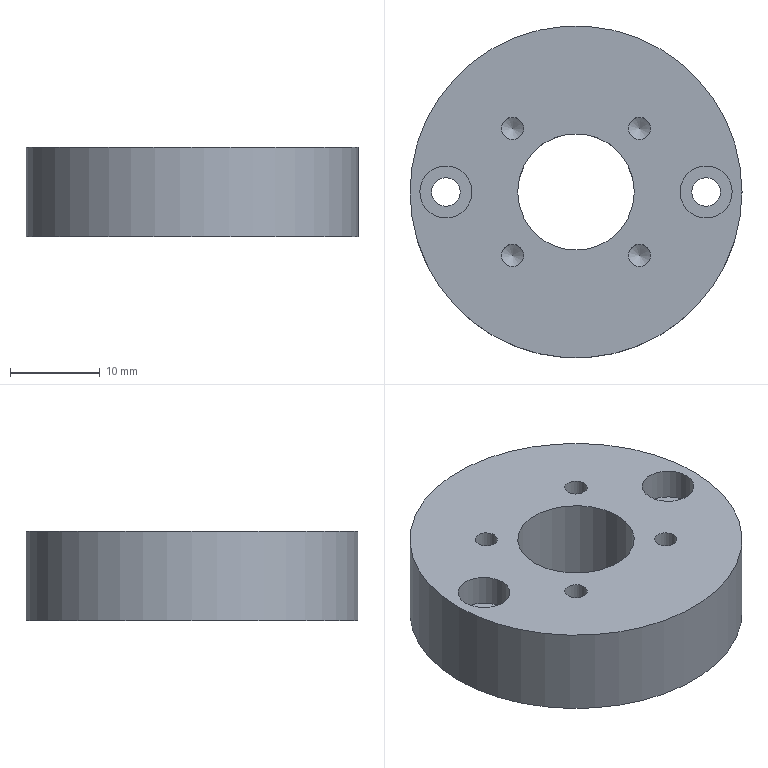Part | NX | 1 solid | 18 faces | box 37 x 37 x 10 mm | volume 8963 mm3 | cylinder 10 | plane 4 | cone 4 | commonest cylinder face diameters 2.5 x4 3.2 x2 5.8 x2 13 x1 37 x1
STEP:
#1=CARTESIAN_POINT('',(18.5,0.,5.));
#2=VERTEX_POINT('',#1);
#3=CARTESIAN_POINT('',(0.,0.,5.));
#4=DIRECTION('',(0.,0.,1.));
#5=DIRECTION('',(1.,0.,0.));
#6=AXIS2_PLACEMENT_3D('',#3,#4,#5);
#7=CIRCLE('',#6,18.5);
#8=EDGE_CURVE('',#2,#2,#7,.T.);
#9=ORIENTED_EDGE('',*,*,#8,.F.);
#10=EDGE_LOOP('',(#9));
#11=FACE_BOUND('',#10,.T.);
#12=CARTESIAN_POINT('',(18.5,0.,-5.));
#13=VERTEX_POINT('',#12);
#14=CARTESIAN_POINT('',(0.,0.,-5.));
#15=DIRECTION('',(0.,0.,1.));
#16=DIRECTION('',(1.,0.,0.));
#17=AXIS2_PLACEMENT_3D('',#14,#15,#16);
#18=CIRCLE('',#17,18.5);
#19=EDGE_CURVE('',#13,#13,#18,.T.);
#20=ORIENTED_EDGE('',*,*,#19,.T.);
#21=EDGE_LOOP('',(#20));
#22=FACE_BOUND('',#21,.T.);
#23=CARTESIAN_POINT('',(0.,0.,5.));
#24=DIRECTION('',(0.,0.,-1.));
#25=DIRECTION('',(-1.,0.,0.));
#26=AXIS2_PLACEMENT_3D('',#23,#24,#25);
#27=CYLINDRICAL_SURFACE('',#26,18.5);
#28=ADVANCED_FACE('',(#11,#22),#27,.T.);
#29=CARTESIAN_POINT('',(6.5,0.,5.));
#30=VERTEX_POINT('',#29);
#31=CARTESIAN_POINT('',(0.,0.,5.));
#32=DIRECTION('',(0.,0.,1.));
#33=DIRECTION('',(1.,0.,0.));
#34=AXIS2_PLACEMENT_3D('',#31,#32,#33);
#35=CIRCLE('',#34,6.5);
#36=EDGE_CURVE('',#30,#30,#35,.T.);
#37=ORIENTED_EDGE('',*,*,#36,.F.);
#38=EDGE_LOOP('',(#37));
#39=FACE_BOUND('',#38,.T.);
#40=CARTESIAN_POINT('',(-5.821,-7.071,5.));
#41=VERTEX_POINT('',#40);
#42=CARTESIAN_POINT('',(-7.071,-7.071,5.));
#43=DIRECTION('',(0.,0.,1.));
#44=DIRECTION('',(1.,0.,0.));
#45=AXIS2_PLACEMENT_3D('',#42,#43,#44);
#46=CIRCLE('',#45,1.25);
#47=EDGE_CURVE('',#41,#41,#46,.T.);
#48=ORIENTED_EDGE('',*,*,#47,.F.);
#49=EDGE_LOOP('',(#48));
#50=FACE_BOUND('',#49,.T.);
#51=CARTESIAN_POINT('',(-5.821,7.071,5.));
#52=VERTEX_POINT('',#51);
#53=CARTESIAN_POINT('',(-7.071,7.071,5.));
#54=DIRECTION('',(0.,0.,1.));
#55=DIRECTION('',(1.,0.,0.));
#56=AXIS2_PLACEMENT_3D('',#53,#54,#55);
#57=CIRCLE('',#56,1.25);
#58=EDGE_CURVE('',#52,#52,#57,.T.);
#59=ORIENTED_EDGE('',*,*,#58,.F.);
#60=EDGE_LOOP('',(#59));
#61=FACE_BOUND('',#60,.T.);
#62=CARTESIAN_POINT('',(8.321,-7.071,5.));
#63=VERTEX_POINT('',#62);
#64=CARTESIAN_POINT('',(7.071,-7.071,5.));
#65=DIRECTION('',(0.,0.,1.));
#66=DIRECTION('',(1.,0.,0.));
#67=AXIS2_PLACEMENT_3D('',#64,#65,#66);
#68=CIRCLE('',#67,1.25);
#69=EDGE_CURVE('',#63,#63,#68,.T.);
#70=ORIENTED_EDGE('',*,*,#69,.F.);
#71=EDGE_LOOP('',(#70));
#72=FACE_BOUND('',#71,.T.);
#73=CARTESIAN_POINT('',(8.321,7.071,5.));
#74=VERTEX_POINT('',#73);
#75=CARTESIAN_POINT('',(7.071,7.071,5.));
#76=DIRECTION('',(0.,0.,1.));
#77=DIRECTION('',(1.,0.,0.));
#78=AXIS2_PLACEMENT_3D('',#75,#76,#77);
#79=CIRCLE('',#78,1.25);
#80=EDGE_CURVE('',#74,#74,#79,.T.);
#81=ORIENTED_EDGE('',*,*,#80,.F.);
#82=EDGE_LOOP('',(#81));
#83=FACE_BOUND('',#82,.T.);
#84=CARTESIAN_POINT('',(-11.6,0.,5.));
#85=VERTEX_POINT('',#84);
#86=CARTESIAN_POINT('',(-14.5,0.,5.));
#87=DIRECTION('',(0.,0.,1.));
#88=DIRECTION('',(1.,0.,0.));
#89=AXIS2_PLACEMENT_3D('',#86,#87,#88);
#90=CIRCLE('',#89,2.9);
#91=EDGE_CURVE('',#85,#85,#90,.T.);
#92=ORIENTED_EDGE('',*,*,#91,.F.);
#93=EDGE_LOOP('',(#92));
#94=FACE_BOUND('',#93,.T.);
#95=CARTESIAN_POINT('',(17.4,0.,5.));
#96=VERTEX_POINT('',#95);
#97=CARTESIAN_POINT('',(14.5,0.,5.));
#98=DIRECTION('',(0.,0.,1.));
#99=DIRECTION('',(1.,0.,0.));
#100=AXIS2_PLACEMENT_3D('',#97,#98,#99);
#101=CIRCLE('',#100,2.9);
#102=EDGE_CURVE('',#96,#96,#101,.T.);
#103=ORIENTED_EDGE('',*,*,#102,.F.);
#104=EDGE_LOOP('',(#103));
#105=FACE_BOUND('',#104,.T.);
#106=ORIENTED_EDGE('',*,*,#8,.T.);
#107=EDGE_LOOP('',(#106));
#108=FACE_BOUND('',#107,.T.);
#109=CARTESIAN_POINT('',(0.,0.,5.));
#110=DIRECTION('',(0.,0.,1.));
#111=DIRECTION('',(1.,0.,0.));
#112=AXIS2_PLACEMENT_3D('',#109,#110,#111);
#113=PLANE('',#112);
#114=ADVANCED_FACE('',(#39,#50,#61,#72,#83,#94,#105,#108),#113,.T.);
#115=CARTESIAN_POINT('',(6.5,0.,-5.));
#116=VERTEX_POINT('',#115);
#117=CARTESIAN_POINT('',(0.,0.,-5.));
#118=DIRECTION('',(0.,0.,1.));
#119=DIRECTION('',(1.,0.,0.));
#120=AXIS2_PLACEMENT_3D('',#117,#118,#119);
#121=CIRCLE('',#120,6.5);
#122=EDGE_CURVE('',#116,#116,#121,.T.);
#123=ORIENTED_EDGE('',*,*,#122,.T.);
#124=EDGE_LOOP('',(#123));
#125=FACE_BOUND('',#124,.T.);
#126=CARTESIAN_POINT('',(-12.9,0.,-5.));
#127=VERTEX_POINT('',#126);
#128=CARTESIAN_POINT('',(-14.5,0.,-5.));
#129=DIRECTION('',(0.,0.,1.));
#130=DIRECTION('',(1.,0.,0.));
#131=AXIS2_PLACEMENT_3D('',#128,#129,#130);
#132=CIRCLE('',#131,1.6);
#133=EDGE_CURVE('',#127,#127,#132,.T.);
#134=ORIENTED_EDGE('',*,*,#133,.T.);
#135=EDGE_LOOP('',(#134));
#136=FACE_BOUND('',#135,.T.);
#137=CARTESIAN_POINT('',(16.1,0.,-5.));
#138=VERTEX_POINT('',#137);
#139=CARTESIAN_POINT('',(14.5,0.,-5.));
#140=DIRECTION('',(0.,0.,1.));
#141=DIRECTION('',(1.,0.,0.));
#142=AXIS2_PLACEMENT_3D('',#139,#140,#141);
#143=CIRCLE('',#142,1.6);
#144=EDGE_CURVE('',#138,#138,#143,.T.);
#145=ORIENTED_EDGE('',*,*,#144,.T.);
#146=EDGE_LOOP('',(#145));
#147=FACE_BOUND('',#146,.T.);
#148=ORIENTED_EDGE('',*,*,#19,.F.);
#149=EDGE_LOOP('',(#148));
#150=FACE_BOUND('',#149,.T.);
#151=CARTESIAN_POINT('',(0.,0.,-5.));
#152=DIRECTION('',(0.,0.,1.));
#153=DIRECTION('',(1.,0.,0.));
#154=AXIS2_PLACEMENT_3D('',#151,#152,#153);
#155=PLANE('',#154);
#156=ADVANCED_FACE('',(#125,#136,#147,#150),#155,.F.);
#157=ORIENTED_EDGE('',*,*,#144,.F.);
#158=EDGE_LOOP('',(#157));
#159=FACE_BOUND('',#158,.T.);
#160=CARTESIAN_POINT('',(16.1,0.,1.5));
#161=VERTEX_POINT('',#160);
#162=CARTESIAN_POINT('',(14.5,0.,1.5));
#163=DIRECTION('',(0.,0.,1.));
#164=DIRECTION('',(1.,0.,0.));
#165=AXIS2_PLACEMENT_3D('',#162,#163,#164);
#166=CIRCLE('',#165,1.6);
#167=EDGE_CURVE('',#161,#161,#166,.T.);
#168=ORIENTED_EDGE('',*,*,#167,.T.);
#169=EDGE_LOOP('',(#168));
#170=FACE_BOUND('',#169,.T.);
#171=CARTESIAN_POINT('',(14.5,0.,5.));
#172=DIRECTION('',(0.,0.,1.));
#173=DIRECTION('',(1.,0.,0.));
#174=AXIS2_PLACEMENT_3D('',#171,#172,#173);
#175=CYLINDRICAL_SURFACE('',#174,1.6);
#176=ADVANCED_FACE('',(#159,#170),#175,.F.);
#177=ORIENTED_EDGE('',*,*,#167,.F.);
#178=EDGE_LOOP('',(#177));
#179=FACE_BOUND('',#178,.T.);
#180=CARTESIAN_POINT('',(17.4,0.,1.5));
#181=VERTEX_POINT('',#180);
#182=CARTESIAN_POINT('',(14.5,0.,1.5));
#183=DIRECTION('',(0.,0.,1.));
#184=DIRECTION('',(1.,0.,0.));
#185=AXIS2_PLACEMENT_3D('',#182,#183,#184);
#186=CIRCLE('',#185,2.9);
#187=EDGE_CURVE('',#181,#181,#186,.T.);
#188=ORIENTED_EDGE('',*,*,#187,.T.);
#189=EDGE_LOOP('',(#188));
#190=FACE_BOUND('',#189,.T.);
#191=CARTESIAN_POINT('',(16.1,0.,1.5));
#192=DIRECTION('',(0.,0.,-1.));
#193=DIRECTION('',(-1.,0.,0.));
#194=AXIS2_PLACEMENT_3D('',#191,#192,#193);
#195=PLANE('',#194);
#196=ADVANCED_FACE('',(#179,#190),#195,.F.);
#197=ORIENTED_EDGE('',*,*,#187,.F.);
#198=EDGE_LOOP('',(#197));
#199=FACE_BOUND('',#198,.T.);
#200=ORIENTED_EDGE('',*,*,#102,.T.);
#201=EDGE_LOOP('',(#200));
#202=FACE_BOUND('',#201,.T.);
#203=CARTESIAN_POINT('',(14.5,0.,5.));
#204=DIRECTION('',(0.,0.,1.));
#205=DIRECTION('',(1.,0.,0.));
#206=AXIS2_PLACEMENT_3D('',#203,#204,#205);
#207=CYLINDRICAL_SURFACE('',#206,2.9);
#208=ADVANCED_FACE('',(#199,#202),#207,.F.);
#209=ORIENTED_EDGE('',*,*,#133,.F.);
#210=EDGE_LOOP('',(#209));
#211=FACE_BOUND('',#210,.T.);
#212=CARTESIAN_POINT('',(-12.9,0.,1.5));
#213=VERTEX_POINT('',#212);
#214=CARTESIAN_POINT('',(-14.5,0.,1.5));
#215=DIRECTION('',(0.,0.,1.));
#216=DIRECTION('',(1.,0.,0.));
#217=AXIS2_PLACEMENT_3D('',#214,#215,#216);
#218=CIRCLE('',#217,1.6);
#219=EDGE_CURVE('',#213,#213,#218,.T.);
#220=ORIENTED_EDGE('',*,*,#219,.T.);
#221=EDGE_LOOP('',(#220));
#222=FACE_BOUND('',#221,.T.);
#223=CARTESIAN_POINT('',(-14.5,0.,5.));
#224=DIRECTION('',(0.,0.,1.));
#225=DIRECTION('',(1.,0.,0.));
#226=AXIS2_PLACEMENT_3D('',#223,#224,#225);
#227=CYLINDRICAL_SURFACE('',#226,1.6);
#228=ADVANCED_FACE('',(#211,#222),#227,.F.);
#229=ORIENTED_EDGE('',*,*,#219,.F.);
#230=EDGE_LOOP('',(#229));
#231=FACE_BOUND('',#230,.T.);
#232=CARTESIAN_POINT('',(-11.6,0.,1.5));
#233=VERTEX_POINT('',#232);
#234=CARTESIAN_POINT('',(-14.5,0.,1.5));
#235=DIRECTION('',(0.,0.,1.));
#236=DIRECTION('',(1.,0.,0.));
#237=AXIS2_PLACEMENT_3D('',#234,#235,#236);
#238=CIRCLE('',#237,2.9);
#239=EDGE_CURVE('',#233,#233,#238,.T.);
#240=ORIENTED_EDGE('',*,*,#239,.T.);
#241=EDGE_LOOP('',(#240));
#242=FACE_BOUND('',#241,.T.);
#243=CARTESIAN_POINT('',(-12.9,0.,1.5));
#244=DIRECTION('',(0.,0.,-1.));
#245=DIRECTION('',(-1.,0.,0.));
#246=AXIS2_PLACEMENT_3D('',#243,#244,#245);
#247=PLANE('',#246);
#248=ADVANCED_FACE('',(#231,#242),#247,.F.);
#249=ORIENTED_EDGE('',*,*,#239,.F.);
#250=EDGE_LOOP('',(#249));
#251=FACE_BOUND('',#250,.T.);
#252=ORIENTED_EDGE('',*,*,#91,.T.);
#253=EDGE_LOOP('',(#252));
#254=FACE_BOUND('',#253,.T.);
#255=CARTESIAN_POINT('',(-14.5,0.,5.));
#256=DIRECTION('',(0.,0.,1.));
#257=DIRECTION('',(1.,0.,0.));
#258=AXIS2_PLACEMENT_3D('',#255,#256,#257);
#259=CYLINDRICAL_SURFACE('',#258,2.9);
#260=ADVANCED_FACE('',(#251,#254),#259,.F.);
#261=CARTESIAN_POINT('',(7.071,7.071,-4.251));
#262=VERTEX_POINT('',#261);
#263=VERTEX_LOOP('',#262);
#264=FACE_BOUND('',#263,.T.);
#265=CARTESIAN_POINT('',(8.321,7.071,-3.5));
#266=VERTEX_POINT('',#265);
#267=CARTESIAN_POINT('',(7.071,7.071,-3.5));
#268=DIRECTION('',(0.,0.,1.));
#269=DIRECTION('',(1.,0.,0.));
#270=AXIS2_PLACEMENT_3D('',#267,#268,#269);
#271=CIRCLE('',#270,1.25);
#272=EDGE_CURVE('',#266,#266,#271,.T.);
#273=ORIENTED_EDGE('',*,*,#272,.T.);
#274=EDGE_LOOP('',(#273));
#275=FACE_BOUND('',#274,.T.);
#276=CARTESIAN_POINT('',(7.071,7.071,-3.5));
#277=DIRECTION('',(0.,0.,1.));
#278=DIRECTION('',(1.,0.,0.));
#279=AXIS2_PLACEMENT_3D('',#276,#277,#278);
#280=CONICAL_SURFACE('',#279,1.25,1.03);
#281=ADVANCED_FACE('',(#264,#275),#280,.F.);
#282=ORIENTED_EDGE('',*,*,#272,.F.);
#283=EDGE_LOOP('',(#282));
#284=FACE_BOUND('',#283,.T.);
#285=ORIENTED_EDGE('',*,*,#80,.T.);
#286=EDGE_LOOP('',(#285));
#287=FACE_BOUND('',#286,.T.);
#288=CARTESIAN_POINT('',(7.071,7.071,5.));
#289=DIRECTION('',(0.,0.,1.));
#290=DIRECTION('',(1.,0.,0.));
#291=AXIS2_PLACEMENT_3D('',#288,#289,#290);
#292=CYLINDRICAL_SURFACE('',#291,1.25);
#293=ADVANCED_FACE('',(#284,#287),#292,.F.);
#294=CARTESIAN_POINT('',(7.071,-7.071,-4.251));
#295=VERTEX_POINT('',#294);
#296=VERTEX_LOOP('',#295);
#297=FACE_BOUND('',#296,.T.);
#298=CARTESIAN_POINT('',(8.321,-7.071,-3.5));
#299=VERTEX_POINT('',#298);
#300=CARTESIAN_POINT('',(7.071,-7.071,-3.5));
#301=DIRECTION('',(0.,0.,1.));
#302=DIRECTION('',(1.,0.,0.));
#303=AXIS2_PLACEMENT_3D('',#300,#301,#302);
#304=CIRCLE('',#303,1.25);
#305=EDGE_CURVE('',#299,#299,#304,.T.);
#306=ORIENTED_EDGE('',*,*,#305,.T.);
#307=EDGE_LOOP('',(#306));
#308=FACE_BOUND('',#307,.T.);
#309=CARTESIAN_POINT('',(7.071,-7.071,-3.5));
#310=DIRECTION('',(0.,0.,1.));
#311=DIRECTION('',(1.,0.,0.));
#312=AXIS2_PLACEMENT_3D('',#309,#310,#311);
#313=CONICAL_SURFACE('',#312,1.25,1.03);
#314=ADVANCED_FACE('',(#297,#308),#313,.F.);
#315=ORIENTED_EDGE('',*,*,#305,.F.);
#316=EDGE_LOOP('',(#315));
#317=FACE_BOUND('',#316,.T.);
#318=ORIENTED_EDGE('',*,*,#69,.T.);
#319=EDGE_LOOP('',(#318));
#320=FACE_BOUND('',#319,.T.);
#321=CARTESIAN_POINT('',(7.071,-7.071,5.));
#322=DIRECTION('',(0.,0.,1.));
#323=DIRECTION('',(1.,0.,0.));
#324=AXIS2_PLACEMENT_3D('',#321,#322,#323);
#325=CYLINDRICAL_SURFACE('',#324,1.25);
#326=ADVANCED_FACE('',(#317,#320),#325,.F.);
#327=CARTESIAN_POINT('',(-7.071,7.071,-4.251));
#328=VERTEX_POINT('',#327);
#329=VERTEX_LOOP('',#328);
#330=FACE_BOUND('',#329,.T.);
#331=CARTESIAN_POINT('',(-5.821,7.071,-3.5));
#332=VERTEX_POINT('',#331);
#333=CARTESIAN_POINT('',(-7.071,7.071,-3.5));
#334=DIRECTION('',(0.,0.,1.));
#335=DIRECTION('',(1.,0.,0.));
#336=AXIS2_PLACEMENT_3D('',#333,#334,#335);
#337=CIRCLE('',#336,1.25);
#338=EDGE_CURVE('',#332,#332,#337,.T.);
#339=ORIENTED_EDGE('',*,*,#338,.T.);
#340=EDGE_LOOP('',(#339));
#341=FACE_BOUND('',#340,.T.);
#342=CARTESIAN_POINT('',(-7.071,7.071,-3.5));
#343=DIRECTION('',(0.,0.,1.));
#344=DIRECTION('',(1.,0.,0.));
#345=AXIS2_PLACEMENT_3D('',#342,#343,#344);
#346=CONICAL_SURFACE('',#345,1.25,1.03);
#347=ADVANCED_FACE('',(#330,#341),#346,.F.);
#348=ORIENTED_EDGE('',*,*,#338,.F.);
#349=EDGE_LOOP('',(#348));
#350=FACE_BOUND('',#349,.T.);
#351=ORIENTED_EDGE('',*,*,#58,.T.);
#352=EDGE_LOOP('',(#351));
#353=FACE_BOUND('',#352,.T.);
#354=CARTESIAN_POINT('',(-7.071,7.071,5.));
#355=DIRECTION('',(0.,0.,1.));
#356=DIRECTION('',(1.,0.,0.));
#357=AXIS2_PLACEMENT_3D('',#354,#355,#356);
#358=CYLINDRICAL_SURFACE('',#357,1.25);
#359=ADVANCED_FACE('',(#350,#353),#358,.F.);
#360=CARTESIAN_POINT('',(-7.071,-7.071,-4.251));
#361=VERTEX_POINT('',#360);
#362=VERTEX_LOOP('',#361);
#363=FACE_BOUND('',#362,.T.);
#364=CARTESIAN_POINT('',(-5.821,-7.071,-3.5));
#365=VERTEX_POINT('',#364);
#366=CARTESIAN_POINT('',(-7.071,-7.071,-3.5));
#367=DIRECTION('',(0.,0.,1.));
#368=DIRECTION('',(1.,0.,0.));
#369=AXIS2_PLACEMENT_3D('',#366,#367,#368);
#370=CIRCLE('',#369,1.25);
#371=EDGE_CURVE('',#365,#365,#370,.T.);
#372=ORIENTED_EDGE('',*,*,#371,.T.);
#373=EDGE_LOOP('',(#372));
#374=FACE_BOUND('',#373,.T.);
#375=CARTESIAN_POINT('',(-7.071,-7.071,-3.5));
#376=DIRECTION('',(0.,0.,1.));
#377=DIRECTION('',(1.,0.,0.));
#378=AXIS2_PLACEMENT_3D('',#375,#376,#377);
#379=CONICAL_SURFACE('',#378,1.25,1.03);
#380=ADVANCED_FACE('',(#363,#374),#379,.F.);
#381=ORIENTED_EDGE('',*,*,#371,.F.);
#382=EDGE_LOOP('',(#381));
#383=FACE_BOUND('',#382,.T.);
#384=ORIENTED_EDGE('',*,*,#47,.T.);
#385=EDGE_LOOP('',(#384));
#386=FACE_BOUND('',#385,.T.);
#387=CARTESIAN_POINT('',(-7.071,-7.071,5.));
#388=DIRECTION('',(0.,0.,1.));
#389=DIRECTION('',(1.,0.,0.));
#390=AXIS2_PLACEMENT_3D('',#387,#388,#389);
#391=CYLINDRICAL_SURFACE('',#390,1.25);
#392=ADVANCED_FACE('',(#383,#386),#391,.F.);
#393=ORIENTED_EDGE('',*,*,#122,.F.);
#394=EDGE_LOOP('',(#393));
#395=FACE_BOUND('',#394,.T.);
#396=ORIENTED_EDGE('',*,*,#36,.T.);
#397=EDGE_LOOP('',(#396));
#398=FACE_BOUND('',#397,.T.);
#399=CARTESIAN_POINT('',(0.,0.,-5.));
#400=DIRECTION('',(0.,0.,1.));
#401=DIRECTION('',(1.,0.,0.));
#402=AXIS2_PLACEMENT_3D('',#399,#400,#401);
#403=CYLINDRICAL_SURFACE('',#402,6.5);
#404=ADVANCED_FACE('',(#395,#398),#403,.F.);
#405=CLOSED_SHELL('',(#28,#114,#156,#176,#196,#208,#228,#248,#260,#281,#293,#314,#326,#347,#359,#380,#392,#404));
#406=MANIFOLD_SOLID_BREP('',#405);
#407=(LENGTH_UNIT()NAMED_UNIT(*)SI_UNIT(.MILLI.,.METRE.));
#408=UNCERTAINTY_MEASURE_WITH_UNIT(LENGTH_MEASURE(0.00001),#407,'','');
#409=(NAMED_UNIT(*)PLANE_ANGLE_UNIT()SI_UNIT($,.RADIAN.));
#410=(NAMED_UNIT(*)SI_UNIT($,.STERADIAN.)SOLID_ANGLE_UNIT());
#411=(GEOMETRIC_REPRESENTATION_CONTEXT(3)GLOBAL_UNCERTAINTY_ASSIGNED_CONTEXT((#408))GLOBAL_UNIT_ASSIGNED_CONTEXT((#407,#409,#410))REPRESENTATION_CONTEXT('',''));
#412=ADVANCED_BREP_SHAPE_REPRESENTATION('',(#406),#411);